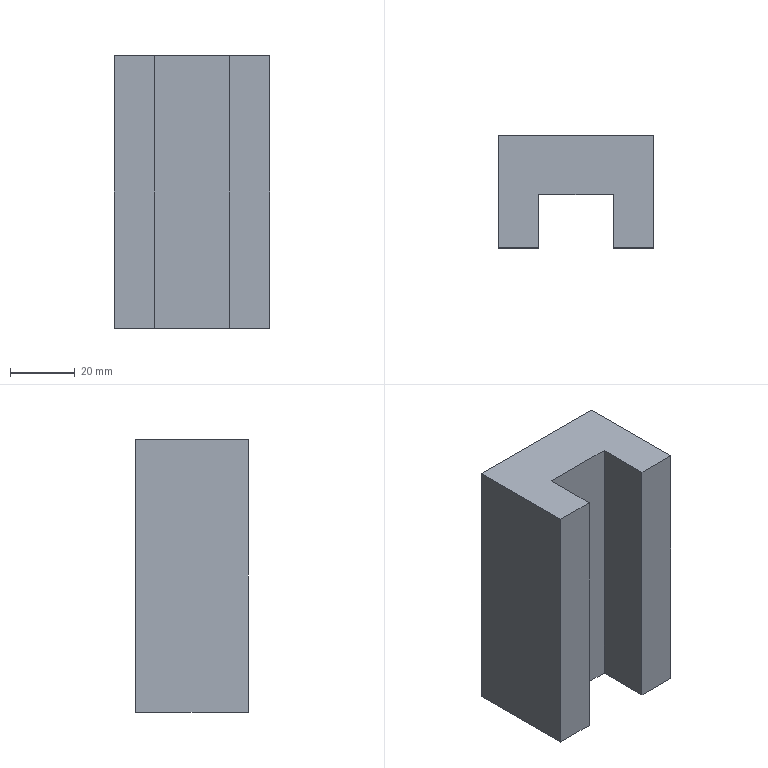Part | SolidWorks | features Extrusion 1, HoleWzd 1 | 1 solid | 26 faces | box 48 x 34.5 x 84 mm | volume 106558 mm3 | plane 10 | cylinder 8 | cone 8 | commonest cylinder face diameters 5 x8
STEP:
#1=CARTESIAN_POINT('',(-17.5,9.25,-20.));
#2=VERTEX_POINT('',#1);
#3=CARTESIAN_POINT('',(-17.5,9.25,-15.));
#4=VERTEX_POINT('',#3);
#5=CARTESIAN_POINT('',(-17.5,9.25,-17.5));
#6=DIRECTION('',(0.,1.,0.));
#7=DIRECTION('',(0.,0.,1.));
#8=AXIS2_PLACEMENT_3D('',#5,#6,#7);
#9=CIRCLE('',#8,2.5);
#10=EDGE_CURVE('',#2,#4,#9,.T.);
#11=ORIENTED_EDGE('',*,*,#10,.F.);
#12=CARTESIAN_POINT('',(-17.5,17.25,-20.));
#13=VERTEX_POINT('',#12);
#14=CARTESIAN_POINT('',(-17.5,17.25,-20.));
#15=DIRECTION('',(0.,1.,0.));
#16=VECTOR('',#15,1000.);
#17=LINE('',#14,#16);
#18=EDGE_CURVE('',#2,#13,#17,.T.);
#19=ORIENTED_EDGE('',*,*,#18,.T.);
#20=CARTESIAN_POINT('',(-17.5,17.25,-15.));
#21=VERTEX_POINT('',#20);
#22=CARTESIAN_POINT('',(-17.5,17.25,-17.5));
#23=DIRECTION('',(0.,1.,0.));
#24=DIRECTION('',(0.,0.,1.));
#25=AXIS2_PLACEMENT_3D('',#22,#23,#24);
#26=CIRCLE('',#25,2.5);
#27=EDGE_CURVE('',#13,#21,#26,.T.);
#28=ORIENTED_EDGE('',*,*,#27,.T.);
#29=CARTESIAN_POINT('',(-17.5,17.25,-15.));
#30=DIRECTION('',(0.,1.,0.));
#31=VECTOR('',#30,1000.);
#32=LINE('',#29,#31);
#33=EDGE_CURVE('',#4,#21,#32,.T.);
#34=ORIENTED_EDGE('',*,*,#33,.F.);
#35=EDGE_LOOP('',(#11,#19,#28,#34));
#36=FACE_OUTER_BOUND('',#35,.T.);
#37=CARTESIAN_POINT('',(-17.5,17.25,-17.5));
#38=DIRECTION('',(0.,1.,0.));
#39=DIRECTION('',(0.,0.,1.));
#40=AXIS2_PLACEMENT_3D('',#37,#38,#39);
#41=CYLINDRICAL_SURFACE('',#40,2.5);
#42=ADVANCED_FACE('',(#36),#41,.F.);
#43=CARTESIAN_POINT('',(-17.5,7.748,-17.5));
#44=VERTEX_POINT('',#43);
#45=CARTESIAN_POINT('',(-17.5,9.25,-15.));
#46=DIRECTION('',(0.,0.515,0.8572));
#47=VECTOR('',#46,1000.);
#48=LINE('',#45,#47);
#49=EDGE_CURVE('',#44,#4,#48,.T.);
#50=ORIENTED_EDGE('',*,*,#49,.F.);
#51=CARTESIAN_POINT('',(-17.5,9.25,-20.));
#52=DIRECTION('',(0.,0.515,-0.8572));
#53=VECTOR('',#52,1000.);
#54=LINE('',#51,#53);
#55=EDGE_CURVE('',#44,#2,#54,.T.);
#56=ORIENTED_EDGE('',*,*,#55,.T.);
#57=ORIENTED_EDGE('',*,*,#10,.T.);
#58=EDGE_LOOP('',(#50,#56,#57));
#59=FACE_OUTER_BOUND('',#58,.T.);
#60=CARTESIAN_POINT('',(-17.5,9.25,-17.5));
#61=DIRECTION('',(0.,1.,0.));
#62=DIRECTION('',(0.,0.,1.));
#63=AXIS2_PLACEMENT_3D('',#60,#61,#62);
#64=CONICAL_SURFACE('',#63,2.5,1.03);
#65=ADVANCED_FACE('',(#59),#64,.F.);
#66=CARTESIAN_POINT('',(17.5,9.25,-20.));
#67=VERTEX_POINT('',#66);
#68=CARTESIAN_POINT('',(17.5,9.25,-15.));
#69=VERTEX_POINT('',#68);
#70=CARTESIAN_POINT('',(17.5,9.25,-17.5));
#71=DIRECTION('',(0.,1.,0.));
#72=DIRECTION('',(0.,0.,1.));
#73=AXIS2_PLACEMENT_3D('',#70,#71,#72);
#74=CIRCLE('',#73,2.5);
#75=EDGE_CURVE('',#67,#69,#74,.T.);
#76=ORIENTED_EDGE('',*,*,#75,.F.);
#77=CARTESIAN_POINT('',(17.5,17.25,-20.));
#78=VERTEX_POINT('',#77);
#79=CARTESIAN_POINT('',(17.5,17.25,-20.));
#80=DIRECTION('',(0.,1.,0.));
#81=VECTOR('',#80,1000.);
#82=LINE('',#79,#81);
#83=EDGE_CURVE('',#67,#78,#82,.T.);
#84=ORIENTED_EDGE('',*,*,#83,.T.);
#85=CARTESIAN_POINT('',(17.5,17.25,-15.));
#86=VERTEX_POINT('',#85);
#87=CARTESIAN_POINT('',(17.5,17.25,-17.5));
#88=DIRECTION('',(0.,1.,0.));
#89=DIRECTION('',(0.,0.,1.));
#90=AXIS2_PLACEMENT_3D('',#87,#88,#89);
#91=CIRCLE('',#90,2.5);
#92=EDGE_CURVE('',#78,#86,#91,.T.);
#93=ORIENTED_EDGE('',*,*,#92,.T.);
#94=CARTESIAN_POINT('',(17.5,17.25,-15.));
#95=DIRECTION('',(0.,1.,0.));
#96=VECTOR('',#95,1000.);
#97=LINE('',#94,#96);
#98=EDGE_CURVE('',#69,#86,#97,.T.);
#99=ORIENTED_EDGE('',*,*,#98,.F.);
#100=EDGE_LOOP('',(#76,#84,#93,#99));
#101=FACE_OUTER_BOUND('',#100,.T.);
#102=CARTESIAN_POINT('',(17.5,17.25,-17.5));
#103=DIRECTION('',(0.,1.,0.));
#104=DIRECTION('',(0.,0.,1.));
#105=AXIS2_PLACEMENT_3D('',#102,#103,#104);
#106=CYLINDRICAL_SURFACE('',#105,2.5);
#107=ADVANCED_FACE('',(#101),#106,.F.);
#108=CARTESIAN_POINT('',(17.5,7.748,-17.5));
#109=VERTEX_POINT('',#108);
#110=CARTESIAN_POINT('',(17.5,9.25,-15.));
#111=DIRECTION('',(0.,0.515,0.8572));
#112=VECTOR('',#111,1000.);
#113=LINE('',#110,#112);
#114=EDGE_CURVE('',#109,#69,#113,.T.);
#115=ORIENTED_EDGE('',*,*,#114,.F.);
#116=CARTESIAN_POINT('',(17.5,9.25,-20.));
#117=DIRECTION('',(0.,0.515,-0.8572));
#118=VECTOR('',#117,1000.);
#119=LINE('',#116,#118);
#120=EDGE_CURVE('',#109,#67,#119,.T.);
#121=ORIENTED_EDGE('',*,*,#120,.T.);
#122=ORIENTED_EDGE('',*,*,#75,.T.);
#123=EDGE_LOOP('',(#115,#121,#122));
#124=FACE_OUTER_BOUND('',#123,.T.);
#125=CARTESIAN_POINT('',(17.5,9.25,-17.5));
#126=DIRECTION('',(0.,1.,0.));
#127=DIRECTION('',(0.,0.,1.));
#128=AXIS2_PLACEMENT_3D('',#125,#126,#127);
#129=CONICAL_SURFACE('',#128,2.5,1.03);
#130=ADVANCED_FACE('',(#124),#129,.F.);
#131=CARTESIAN_POINT('',(17.5,9.25,15.));
#132=VERTEX_POINT('',#131);
#133=CARTESIAN_POINT('',(17.5,9.25,20.));
#134=VERTEX_POINT('',#133);
#135=CARTESIAN_POINT('',(17.5,9.25,17.5));
#136=DIRECTION('',(0.,1.,0.));
#137=DIRECTION('',(0.,0.,1.));
#138=AXIS2_PLACEMENT_3D('',#135,#136,#137);
#139=CIRCLE('',#138,2.5);
#140=EDGE_CURVE('',#132,#134,#139,.T.);
#141=ORIENTED_EDGE('',*,*,#140,.F.);
#142=CARTESIAN_POINT('',(17.5,17.25,15.));
#143=VERTEX_POINT('',#142);
#144=CARTESIAN_POINT('',(17.5,17.25,15.));
#145=DIRECTION('',(0.,1.,0.));
#146=VECTOR('',#145,1000.);
#147=LINE('',#144,#146);
#148=EDGE_CURVE('',#132,#143,#147,.T.);
#149=ORIENTED_EDGE('',*,*,#148,.T.);
#150=CARTESIAN_POINT('',(17.5,17.25,20.));
#151=VERTEX_POINT('',#150);
#152=CARTESIAN_POINT('',(17.5,17.25,17.5));
#153=DIRECTION('',(0.,1.,0.));
#154=DIRECTION('',(0.,0.,1.));
#155=AXIS2_PLACEMENT_3D('',#152,#153,#154);
#156=CIRCLE('',#155,2.5);
#157=EDGE_CURVE('',#143,#151,#156,.T.);
#158=ORIENTED_EDGE('',*,*,#157,.T.);
#159=CARTESIAN_POINT('',(17.5,17.25,20.));
#160=DIRECTION('',(0.,1.,0.));
#161=VECTOR('',#160,1000.);
#162=LINE('',#159,#161);
#163=EDGE_CURVE('',#134,#151,#162,.T.);
#164=ORIENTED_EDGE('',*,*,#163,.F.);
#165=EDGE_LOOP('',(#141,#149,#158,#164));
#166=FACE_OUTER_BOUND('',#165,.T.);
#167=CARTESIAN_POINT('',(17.5,17.25,17.5));
#168=DIRECTION('',(0.,1.,0.));
#169=DIRECTION('',(0.,0.,1.));
#170=AXIS2_PLACEMENT_3D('',#167,#168,#169);
#171=CYLINDRICAL_SURFACE('',#170,2.5);
#172=ADVANCED_FACE('',(#166),#171,.F.);
#173=CARTESIAN_POINT('',(17.5,7.748,17.5));
#174=VERTEX_POINT('',#173);
#175=CARTESIAN_POINT('',(17.5,9.25,20.));
#176=DIRECTION('',(0.,0.515,0.8572));
#177=VECTOR('',#176,1000.);
#178=LINE('',#175,#177);
#179=EDGE_CURVE('',#174,#134,#178,.T.);
#180=ORIENTED_EDGE('',*,*,#179,.F.);
#181=CARTESIAN_POINT('',(17.5,9.25,15.));
#182=DIRECTION('',(0.,0.515,-0.8572));
#183=VECTOR('',#182,1000.);
#184=LINE('',#181,#183);
#185=EDGE_CURVE('',#174,#132,#184,.T.);
#186=ORIENTED_EDGE('',*,*,#185,.T.);
#187=ORIENTED_EDGE('',*,*,#140,.T.);
#188=EDGE_LOOP('',(#180,#186,#187));
#189=FACE_OUTER_BOUND('',#188,.T.);
#190=CARTESIAN_POINT('',(17.5,9.25,17.5));
#191=DIRECTION('',(0.,1.,0.));
#192=DIRECTION('',(0.,0.,1.));
#193=AXIS2_PLACEMENT_3D('',#190,#191,#192);
#194=CONICAL_SURFACE('',#193,2.5,1.03);
#195=ADVANCED_FACE('',(#189),#194,.F.);
#196=CARTESIAN_POINT('',(-17.5,9.25,15.));
#197=VERTEX_POINT('',#196);
#198=CARTESIAN_POINT('',(-17.5,9.25,20.));
#199=VERTEX_POINT('',#198);
#200=CARTESIAN_POINT('',(-17.5,9.25,17.5));
#201=DIRECTION('',(0.,1.,0.));
#202=DIRECTION('',(0.,0.,1.));
#203=AXIS2_PLACEMENT_3D('',#200,#201,#202);
#204=CIRCLE('',#203,2.5);
#205=EDGE_CURVE('',#197,#199,#204,.T.);
#206=ORIENTED_EDGE('',*,*,#205,.F.);
#207=CARTESIAN_POINT('',(-17.5,17.25,15.));
#208=VERTEX_POINT('',#207);
#209=CARTESIAN_POINT('',(-17.5,17.25,15.));
#210=DIRECTION('',(0.,1.,0.));
#211=VECTOR('',#210,1000.);
#212=LINE('',#209,#211);
#213=EDGE_CURVE('',#197,#208,#212,.T.);
#214=ORIENTED_EDGE('',*,*,#213,.T.);
#215=CARTESIAN_POINT('',(-17.5,17.25,20.));
#216=VERTEX_POINT('',#215);
#217=CARTESIAN_POINT('',(-17.5,17.25,17.5));
#218=DIRECTION('',(0.,1.,0.));
#219=DIRECTION('',(0.,0.,1.));
#220=AXIS2_PLACEMENT_3D('',#217,#218,#219);
#221=CIRCLE('',#220,2.5);
#222=EDGE_CURVE('',#208,#216,#221,.T.);
#223=ORIENTED_EDGE('',*,*,#222,.T.);
#224=CARTESIAN_POINT('',(-17.5,17.25,20.));
#225=DIRECTION('',(0.,1.,0.));
#226=VECTOR('',#225,1000.);
#227=LINE('',#224,#226);
#228=EDGE_CURVE('',#199,#216,#227,.T.);
#229=ORIENTED_EDGE('',*,*,#228,.F.);
#230=EDGE_LOOP('',(#206,#214,#223,#229));
#231=FACE_OUTER_BOUND('',#230,.T.);
#232=CARTESIAN_POINT('',(-17.5,17.25,17.5));
#233=DIRECTION('',(0.,1.,0.));
#234=DIRECTION('',(0.,0.,1.));
#235=AXIS2_PLACEMENT_3D('',#232,#233,#234);
#236=CYLINDRICAL_SURFACE('',#235,2.5);
#237=ADVANCED_FACE('',(#231),#236,.F.);
#238=CARTESIAN_POINT('',(-17.5,7.748,17.5));
#239=VERTEX_POINT('',#238);
#240=CARTESIAN_POINT('',(-17.5,9.25,20.));
#241=DIRECTION('',(0.,0.515,0.8572));
#242=VECTOR('',#241,1000.);
#243=LINE('',#240,#242);
#244=EDGE_CURVE('',#239,#199,#243,.T.);
#245=ORIENTED_EDGE('',*,*,#244,.F.);
#246=CARTESIAN_POINT('',(-17.5,9.25,15.));
#247=DIRECTION('',(0.,0.515,-0.8572));
#248=VECTOR('',#247,1000.);
#249=LINE('',#246,#248);
#250=EDGE_CURVE('',#239,#197,#249,.T.);
#251=ORIENTED_EDGE('',*,*,#250,.T.);
#252=ORIENTED_EDGE('',*,*,#205,.T.);
#253=EDGE_LOOP('',(#245,#251,#252));
#254=FACE_OUTER_BOUND('',#253,.T.);
#255=CARTESIAN_POINT('',(-17.5,9.25,17.5));
#256=DIRECTION('',(0.,1.,0.));
#257=DIRECTION('',(0.,0.,1.));
#258=AXIS2_PLACEMENT_3D('',#255,#256,#257);
#259=CONICAL_SURFACE('',#258,2.5,1.03);
#260=ADVANCED_FACE('',(#254),#259,.F.);
#261=CARTESIAN_POINT('',(-24.,17.25,-42.));
#262=VERTEX_POINT('',#261);
#263=CARTESIAN_POINT('',(-24.,-17.25,-42.));
#264=VERTEX_POINT('',#263);
#265=CARTESIAN_POINT('',(-24.,-17.25,-42.));
#266=DIRECTION('',(0.,-1.,0.));
#267=VECTOR('',#266,1000.);
#268=LINE('',#265,#267);
#269=EDGE_CURVE('',#262,#264,#268,.T.);
#270=ORIENTED_EDGE('',*,*,#269,.T.);
#271=CARTESIAN_POINT('',(-24.,-17.25,42.));
#272=VERTEX_POINT('',#271);
#273=CARTESIAN_POINT('',(-24.,-17.25,42.));
#274=DIRECTION('',(0.,0.,-1.));
#275=VECTOR('',#274,1000.);
#276=LINE('',#273,#275);
#277=EDGE_CURVE('',#272,#264,#276,.T.);
#278=ORIENTED_EDGE('',*,*,#277,.F.);
#279=CARTESIAN_POINT('',(-24.,17.25,42.));
#280=VERTEX_POINT('',#279);
#281=CARTESIAN_POINT('',(-24.,-17.25,42.));
#282=DIRECTION('',(0.,-1.,0.));
#283=VECTOR('',#282,1000.);
#284=LINE('',#281,#283);
#285=EDGE_CURVE('',#280,#272,#284,.T.);
#286=ORIENTED_EDGE('',*,*,#285,.F.);
#287=CARTESIAN_POINT('',(-24.,17.25,42.));
#288=DIRECTION('',(0.,0.,-1.));
#289=VECTOR('',#288,1000.);
#290=LINE('',#287,#289);
#291=EDGE_CURVE('',#280,#262,#290,.T.);
#292=ORIENTED_EDGE('',*,*,#291,.T.);
#293=EDGE_LOOP('',(#270,#278,#286,#292));
#294=FACE_OUTER_BOUND('',#293,.T.);
#295=CARTESIAN_POINT('',(-24.,-17.25,42.));
#296=DIRECTION('',(1.,0.,0.));
#297=DIRECTION('',(0.,0.,-1.));
#298=AXIS2_PLACEMENT_3D('',#295,#296,#297);
#299=PLANE('',#298);
#300=ADVANCED_FACE('',(#294),#299,.F.);
#301=CARTESIAN_POINT('',(-11.5,-17.25,-42.));
#302=VERTEX_POINT('',#301);
#303=CARTESIAN_POINT('',(-11.5,-17.25,-42.));
#304=DIRECTION('',(1.,0.,0.));
#305=VECTOR('',#304,1000.);
#306=LINE('',#303,#305);
#307=EDGE_CURVE('',#264,#302,#306,.T.);
#308=ORIENTED_EDGE('',*,*,#307,.T.);
#309=CARTESIAN_POINT('',(-11.5,-17.25,42.));
#310=VERTEX_POINT('',#309);
#311=CARTESIAN_POINT('',(-11.5,-17.25,42.));
#312=DIRECTION('',(0.,0.,-1.));
#313=VECTOR('',#312,1000.);
#314=LINE('',#311,#313);
#315=EDGE_CURVE('',#310,#302,#314,.T.);
#316=ORIENTED_EDGE('',*,*,#315,.F.);
#317=CARTESIAN_POINT('',(-11.5,-17.25,42.));
#318=DIRECTION('',(1.,0.,0.));
#319=VECTOR('',#318,1000.);
#320=LINE('',#317,#319);
#321=EDGE_CURVE('',#272,#310,#320,.T.);
#322=ORIENTED_EDGE('',*,*,#321,.F.);
#323=ORIENTED_EDGE('',*,*,#277,.T.);
#324=EDGE_LOOP('',(#308,#316,#322,#323));
#325=FACE_OUTER_BOUND('',#324,.T.);
#326=CARTESIAN_POINT('',(-11.5,-17.25,42.));
#327=DIRECTION('',(0.,1.,0.));
#328=DIRECTION('',(0.,0.,1.));
#329=AXIS2_PLACEMENT_3D('',#326,#327,#328);
#330=PLANE('',#329);
#331=ADVANCED_FACE('',(#325),#330,.F.);
#332=CARTESIAN_POINT('',(-11.5,-0.75,-42.));
#333=VERTEX_POINT('',#332);
#334=CARTESIAN_POINT('',(-11.5,-0.75,-42.));
#335=DIRECTION('',(0.,1.,0.));
#336=VECTOR('',#335,1000.);
#337=LINE('',#334,#336);
#338=EDGE_CURVE('',#302,#333,#337,.T.);
#339=ORIENTED_EDGE('',*,*,#338,.T.);
#340=CARTESIAN_POINT('',(-11.5,-0.75,42.));
#341=VERTEX_POINT('',#340);
#342=CARTESIAN_POINT('',(-11.5,-0.75,42.));
#343=DIRECTION('',(0.,0.,-1.));
#344=VECTOR('',#343,1000.);
#345=LINE('',#342,#344);
#346=EDGE_CURVE('',#341,#333,#345,.T.);
#347=ORIENTED_EDGE('',*,*,#346,.F.);
#348=CARTESIAN_POINT('',(-11.5,-0.75,42.));
#349=DIRECTION('',(0.,1.,0.));
#350=VECTOR('',#349,1000.);
#351=LINE('',#348,#350);
#352=EDGE_CURVE('',#310,#341,#351,.T.);
#353=ORIENTED_EDGE('',*,*,#352,.F.);
#354=ORIENTED_EDGE('',*,*,#315,.T.);
#355=EDGE_LOOP('',(#339,#347,#353,#354));
#356=FACE_OUTER_BOUND('',#355,.T.);
#357=CARTESIAN_POINT('',(-11.5,-0.75,42.));
#358=DIRECTION('',(-1.,0.,0.));
#359=DIRECTION('',(0.,-1.,0.));
#360=AXIS2_PLACEMENT_3D('',#357,#358,#359);
#361=PLANE('',#360);
#362=ADVANCED_FACE('',(#356),#361,.F.);
#363=CARTESIAN_POINT('',(11.5,-0.75,-42.));
#364=VERTEX_POINT('',#363);
#365=CARTESIAN_POINT('',(-11.5,-0.75,-42.));
#366=DIRECTION('',(1.,0.,0.));
#367=VECTOR('',#366,1000.);
#368=LINE('',#365,#367);
#369=EDGE_CURVE('',#333,#364,#368,.T.);
#370=ORIENTED_EDGE('',*,*,#369,.T.);
#371=CARTESIAN_POINT('',(11.5,-0.75,42.));
#372=VERTEX_POINT('',#371);
#373=CARTESIAN_POINT('',(11.5,-0.75,42.));
#374=DIRECTION('',(0.,0.,-1.));
#375=VECTOR('',#374,1000.);
#376=LINE('',#373,#375);
#377=EDGE_CURVE('',#372,#364,#376,.T.);
#378=ORIENTED_EDGE('',*,*,#377,.F.);
#379=CARTESIAN_POINT('',(-11.5,-0.75,42.));
#380=DIRECTION('',(1.,0.,0.));
#381=VECTOR('',#380,1000.);
#382=LINE('',#379,#381);
#383=EDGE_CURVE('',#341,#372,#382,.T.);
#384=ORIENTED_EDGE('',*,*,#383,.F.);
#385=ORIENTED_EDGE('',*,*,#346,.T.);
#386=EDGE_LOOP('',(#370,#378,#384,#385));
#387=FACE_OUTER_BOUND('',#386,.T.);
#388=CARTESIAN_POINT('',(-11.5,-0.75,42.));
#389=DIRECTION('',(0.,1.,0.));
#390=DIRECTION('',(-1.,0.,0.));
#391=AXIS2_PLACEMENT_3D('',#388,#389,#390);
#392=PLANE('',#391);
#393=ADVANCED_FACE('',(#387),#392,.F.);
#394=CARTESIAN_POINT('',(11.5,-17.25,-42.));
#395=VERTEX_POINT('',#394);
#396=CARTESIAN_POINT('',(11.5,-0.75,-42.));
#397=DIRECTION('',(0.,-1.,0.));
#398=VECTOR('',#397,1000.);
#399=LINE('',#396,#398);
#400=EDGE_CURVE('',#364,#395,#399,.T.);
#401=ORIENTED_EDGE('',*,*,#400,.T.);
#402=CARTESIAN_POINT('',(11.5,-17.25,42.));
#403=VERTEX_POINT('',#402);
#404=CARTESIAN_POINT('',(11.5,-17.25,42.));
#405=DIRECTION('',(0.,0.,-1.));
#406=VECTOR('',#405,1000.);
#407=LINE('',#404,#406);
#408=EDGE_CURVE('',#403,#395,#407,.T.);
#409=ORIENTED_EDGE('',*,*,#408,.F.);
#410=CARTESIAN_POINT('',(11.5,-0.75,42.));
#411=DIRECTION('',(0.,-1.,0.));
#412=VECTOR('',#411,1000.);
#413=LINE('',#410,#412);
#414=EDGE_CURVE('',#372,#403,#413,.T.);
#415=ORIENTED_EDGE('',*,*,#414,.F.);
#416=ORIENTED_EDGE('',*,*,#377,.T.);
#417=EDGE_LOOP('',(#401,#409,#415,#416));
#418=FACE_OUTER_BOUND('',#417,.T.);
#419=CARTESIAN_POINT('',(11.5,-0.75,42.));
#420=DIRECTION('',(1.,0.,0.));
#421=DIRECTION('',(0.,1.,0.));
#422=AXIS2_PLACEMENT_3D('',#419,#420,#421);
#423=PLANE('',#422);
#424=ADVANCED_FACE('',(#418),#423,.F.);
#425=CARTESIAN_POINT('',(24.,-17.25,-42.));
#426=VERTEX_POINT('',#425);
#427=CARTESIAN_POINT('',(24.,-17.25,-42.));
#428=DIRECTION('',(1.,0.,0.));
#429=VECTOR('',#428,1000.);
#430=LINE('',#427,#429);
#431=EDGE_CURVE('',#395,#426,#430,.T.);
#432=ORIENTED_EDGE('',*,*,#431,.T.);
#433=CARTESIAN_POINT('',(24.,-17.25,42.));
#434=VERTEX_POINT('',#433);
#435=CARTESIAN_POINT('',(24.,-17.25,42.));
#436=DIRECTION('',(0.,0.,-1.));
#437=VECTOR('',#436,1000.);
#438=LINE('',#435,#437);
#439=EDGE_CURVE('',#434,#426,#438,.T.);
#440=ORIENTED_EDGE('',*,*,#439,.F.);
#441=CARTESIAN_POINT('',(24.,-17.25,42.));
#442=DIRECTION('',(1.,0.,0.));
#443=VECTOR('',#442,1000.);
#444=LINE('',#441,#443);
#445=EDGE_CURVE('',#403,#434,#444,.T.);
#446=ORIENTED_EDGE('',*,*,#445,.F.);
#447=ORIENTED_EDGE('',*,*,#408,.T.);
#448=EDGE_LOOP('',(#432,#440,#446,#447));
#449=FACE_OUTER_BOUND('',#448,.T.);
#450=CARTESIAN_POINT('',(24.,-17.25,42.));
#451=DIRECTION('',(0.,1.,0.));
#452=DIRECTION('',(-1.,0.,0.));
#453=AXIS2_PLACEMENT_3D('',#450,#451,#452);
#454=PLANE('',#453);
#455=ADVANCED_FACE('',(#449),#454,.F.);
#456=CARTESIAN_POINT('',(24.,17.25,-42.));
#457=VERTEX_POINT('',#456);
#458=CARTESIAN_POINT('',(24.,-17.25,-42.));
#459=DIRECTION('',(0.,1.,0.));
#460=VECTOR('',#459,1000.);
#461=LINE('',#458,#460);
#462=EDGE_CURVE('',#426,#457,#461,.T.);
#463=ORIENTED_EDGE('',*,*,#462,.T.);
#464=CARTESIAN_POINT('',(24.,17.25,42.));
#465=VERTEX_POINT('',#464);
#466=CARTESIAN_POINT('',(24.,17.25,42.));
#467=DIRECTION('',(0.,0.,-1.));
#468=VECTOR('',#467,1000.);
#469=LINE('',#466,#468);
#470=EDGE_CURVE('',#465,#457,#469,.T.);
#471=ORIENTED_EDGE('',*,*,#470,.F.);
#472=CARTESIAN_POINT('',(24.,-17.25,42.));
#473=DIRECTION('',(0.,1.,0.));
#474=VECTOR('',#473,1000.);
#475=LINE('',#472,#474);
#476=EDGE_CURVE('',#434,#465,#475,.T.);
#477=ORIENTED_EDGE('',*,*,#476,.F.);
#478=ORIENTED_EDGE('',*,*,#439,.T.);
#479=EDGE_LOOP('',(#463,#471,#477,#478));
#480=FACE_OUTER_BOUND('',#479,.T.);
#481=CARTESIAN_POINT('',(24.,-17.25,42.));
#482=DIRECTION('',(-1.,0.,0.));
#483=DIRECTION('',(0.,0.,1.));
#484=AXIS2_PLACEMENT_3D('',#481,#482,#483);
#485=PLANE('',#484);
#486=ADVANCED_FACE('',(#480),#485,.F.);
#487=CARTESIAN_POINT('',(-17.5,17.25,-17.5));
#488=DIRECTION('',(0.,1.,0.));
#489=DIRECTION('',(0.,0.,1.));
#490=AXIS2_PLACEMENT_3D('',#487,#488,#489);
#491=CIRCLE('',#490,2.5);
#492=EDGE_CURVE('',#21,#13,#491,.T.);
#493=ORIENTED_EDGE('',*,*,#492,.F.);
#494=ORIENTED_EDGE('',*,*,#27,.F.);
#495=EDGE_LOOP('',(#493,#494));
#496=FACE_BOUND('',#495,.T.);
#497=CARTESIAN_POINT('',(17.5,17.25,-17.5));
#498=DIRECTION('',(0.,1.,0.));
#499=DIRECTION('',(0.,0.,1.));
#500=AXIS2_PLACEMENT_3D('',#497,#498,#499);
#501=CIRCLE('',#500,2.5);
#502=EDGE_CURVE('',#86,#78,#501,.T.);
#503=ORIENTED_EDGE('',*,*,#502,.F.);
#504=ORIENTED_EDGE('',*,*,#92,.F.);
#505=EDGE_LOOP('',(#503,#504));
#506=FACE_BOUND('',#505,.T.);
#507=CARTESIAN_POINT('',(17.5,17.25,17.5));
#508=DIRECTION('',(0.,1.,0.));
#509=DIRECTION('',(0.,0.,1.));
#510=AXIS2_PLACEMENT_3D('',#507,#508,#509);
#511=CIRCLE('',#510,2.5);
#512=EDGE_CURVE('',#151,#143,#511,.T.);
#513=ORIENTED_EDGE('',*,*,#512,.F.);
#514=ORIENTED_EDGE('',*,*,#157,.F.);
#515=EDGE_LOOP('',(#513,#514));
#516=FACE_BOUND('',#515,.T.);
#517=CARTESIAN_POINT('',(-17.5,17.25,17.5));
#518=DIRECTION('',(0.,1.,0.));
#519=DIRECTION('',(0.,0.,1.));
#520=AXIS2_PLACEMENT_3D('',#517,#518,#519);
#521=CIRCLE('',#520,2.5);
#522=EDGE_CURVE('',#216,#208,#521,.T.);
#523=ORIENTED_EDGE('',*,*,#522,.F.);
#524=ORIENTED_EDGE('',*,*,#222,.F.);
#525=EDGE_LOOP('',(#523,#524));
#526=FACE_BOUND('',#525,.T.);
#527=CARTESIAN_POINT('',(24.,17.25,-42.));
#528=DIRECTION('',(-1.,0.,0.));
#529=VECTOR('',#528,1000.);
#530=LINE('',#527,#529);
#531=EDGE_CURVE('',#457,#262,#530,.T.);
#532=ORIENTED_EDGE('',*,*,#531,.T.);
#533=ORIENTED_EDGE('',*,*,#291,.F.);
#534=CARTESIAN_POINT('',(24.,17.25,42.));
#535=DIRECTION('',(-1.,0.,0.));
#536=VECTOR('',#535,1000.);
#537=LINE('',#534,#536);
#538=EDGE_CURVE('',#465,#280,#537,.T.);
#539=ORIENTED_EDGE('',*,*,#538,.F.);
#540=ORIENTED_EDGE('',*,*,#470,.T.);
#541=EDGE_LOOP('',(#532,#533,#539,#540));
#542=FACE_OUTER_BOUND('',#541,.T.);
#543=CARTESIAN_POINT('',(24.,17.25,42.));
#544=DIRECTION('',(0.,-1.,0.));
#545=DIRECTION('',(1.,0.,0.));
#546=AXIS2_PLACEMENT_3D('',#543,#544,#545);
#547=PLANE('',#546);
#548=ADVANCED_FACE('',(#496,#506,#516,#526,#542),#547,.F.);
#549=ORIENTED_EDGE('',*,*,#285,.T.);
#550=ORIENTED_EDGE('',*,*,#321,.T.);
#551=ORIENTED_EDGE('',*,*,#352,.T.);
#552=ORIENTED_EDGE('',*,*,#383,.T.);
#553=ORIENTED_EDGE('',*,*,#414,.T.);
#554=ORIENTED_EDGE('',*,*,#445,.T.);
#555=ORIENTED_EDGE('',*,*,#476,.T.);
#556=ORIENTED_EDGE('',*,*,#538,.T.);
#557=EDGE_LOOP('',(#549,#550,#551,#552,#553,#554,#555,#556));
#558=FACE_OUTER_BOUND('',#557,.T.);
#559=CARTESIAN_POINT('',(0.,0.,42.));
#560=DIRECTION('',(0.,0.,1.));
#561=DIRECTION('',(1.,0.,0.));
#562=AXIS2_PLACEMENT_3D('',#559,#560,#561);
#563=PLANE('',#562);
#564=ADVANCED_FACE('',(#558),#563,.T.);
#565=ORIENTED_EDGE('',*,*,#269,.F.);
#566=ORIENTED_EDGE('',*,*,#531,.F.);
#567=ORIENTED_EDGE('',*,*,#462,.F.);
#568=ORIENTED_EDGE('',*,*,#431,.F.);
#569=ORIENTED_EDGE('',*,*,#400,.F.);
#570=ORIENTED_EDGE('',*,*,#369,.F.);
#571=ORIENTED_EDGE('',*,*,#338,.F.);
#572=ORIENTED_EDGE('',*,*,#307,.F.);
#573=EDGE_LOOP('',(#565,#566,#567,#568,#569,#570,#571,#572));
#574=FACE_OUTER_BOUND('',#573,.T.);
#575=CARTESIAN_POINT('',(0.,0.,-42.));
#576=DIRECTION('',(0.,0.,1.));
#577=DIRECTION('',(1.,0.,0.));
#578=AXIS2_PLACEMENT_3D('',#575,#576,#577);
#579=PLANE('',#578);
#580=ADVANCED_FACE('',(#574),#579,.F.);
#581=ORIENTED_EDGE('',*,*,#250,.F.);
#582=ORIENTED_EDGE('',*,*,#244,.T.);
#583=CARTESIAN_POINT('',(-17.5,9.25,17.5));
#584=DIRECTION('',(0.,1.,0.));
#585=DIRECTION('',(0.,0.,1.));
#586=AXIS2_PLACEMENT_3D('',#583,#584,#585);
#587=CIRCLE('',#586,2.5);
#588=EDGE_CURVE('',#199,#197,#587,.T.);
#589=ORIENTED_EDGE('',*,*,#588,.T.);
#590=EDGE_LOOP('',(#581,#582,#589));
#591=FACE_OUTER_BOUND('',#590,.T.);
#592=CARTESIAN_POINT('',(-17.5,9.25,17.5));
#593=DIRECTION('',(0.,1.,0.));
#594=DIRECTION('',(0.,0.,1.));
#595=AXIS2_PLACEMENT_3D('',#592,#593,#594);
#596=CONICAL_SURFACE('',#595,2.5,1.03);
#597=ADVANCED_FACE('',(#591),#596,.F.);
#598=ORIENTED_EDGE('',*,*,#213,.F.);
#599=ORIENTED_EDGE('',*,*,#588,.F.);
#600=ORIENTED_EDGE('',*,*,#228,.T.);
#601=ORIENTED_EDGE('',*,*,#522,.T.);
#602=EDGE_LOOP('',(#598,#599,#600,#601));
#603=FACE_OUTER_BOUND('',#602,.T.);
#604=CARTESIAN_POINT('',(-17.5,17.25,17.5));
#605=DIRECTION('',(0.,1.,0.));
#606=DIRECTION('',(0.,0.,1.));
#607=AXIS2_PLACEMENT_3D('',#604,#605,#606);
#608=CYLINDRICAL_SURFACE('',#607,2.5);
#609=ADVANCED_FACE('',(#603),#608,.F.);
#610=ORIENTED_EDGE('',*,*,#185,.F.);
#611=ORIENTED_EDGE('',*,*,#179,.T.);
#612=CARTESIAN_POINT('',(17.5,9.25,17.5));
#613=DIRECTION('',(0.,1.,0.));
#614=DIRECTION('',(0.,0.,1.));
#615=AXIS2_PLACEMENT_3D('',#612,#613,#614);
#616=CIRCLE('',#615,2.5);
#617=EDGE_CURVE('',#134,#132,#616,.T.);
#618=ORIENTED_EDGE('',*,*,#617,.T.);
#619=EDGE_LOOP('',(#610,#611,#618));
#620=FACE_OUTER_BOUND('',#619,.T.);
#621=CARTESIAN_POINT('',(17.5,9.25,17.5));
#622=DIRECTION('',(0.,1.,0.));
#623=DIRECTION('',(0.,0.,1.));
#624=AXIS2_PLACEMENT_3D('',#621,#622,#623);
#625=CONICAL_SURFACE('',#624,2.5,1.03);
#626=ADVANCED_FACE('',(#620),#625,.F.);
#627=ORIENTED_EDGE('',*,*,#148,.F.);
#628=ORIENTED_EDGE('',*,*,#617,.F.);
#629=ORIENTED_EDGE('',*,*,#163,.T.);
#630=ORIENTED_EDGE('',*,*,#512,.T.);
#631=EDGE_LOOP('',(#627,#628,#629,#630));
#632=FACE_OUTER_BOUND('',#631,.T.);
#633=CARTESIAN_POINT('',(17.5,17.25,17.5));
#634=DIRECTION('',(0.,1.,0.));
#635=DIRECTION('',(0.,0.,1.));
#636=AXIS2_PLACEMENT_3D('',#633,#634,#635);
#637=CYLINDRICAL_SURFACE('',#636,2.5);
#638=ADVANCED_FACE('',(#632),#637,.F.);
#639=ORIENTED_EDGE('',*,*,#120,.F.);
#640=ORIENTED_EDGE('',*,*,#114,.T.);
#641=CARTESIAN_POINT('',(17.5,9.25,-17.5));
#642=DIRECTION('',(0.,1.,0.));
#643=DIRECTION('',(0.,0.,1.));
#644=AXIS2_PLACEMENT_3D('',#641,#642,#643);
#645=CIRCLE('',#644,2.5);
#646=EDGE_CURVE('',#69,#67,#645,.T.);
#647=ORIENTED_EDGE('',*,*,#646,.T.);
#648=EDGE_LOOP('',(#639,#640,#647));
#649=FACE_OUTER_BOUND('',#648,.T.);
#650=CARTESIAN_POINT('',(17.5,9.25,-17.5));
#651=DIRECTION('',(0.,1.,0.));
#652=DIRECTION('',(0.,0.,1.));
#653=AXIS2_PLACEMENT_3D('',#650,#651,#652);
#654=CONICAL_SURFACE('',#653,2.5,1.03);
#655=ADVANCED_FACE('',(#649),#654,.F.);
#656=ORIENTED_EDGE('',*,*,#83,.F.);
#657=ORIENTED_EDGE('',*,*,#646,.F.);
#658=ORIENTED_EDGE('',*,*,#98,.T.);
#659=ORIENTED_EDGE('',*,*,#502,.T.);
#660=EDGE_LOOP('',(#656,#657,#658,#659));
#661=FACE_OUTER_BOUND('',#660,.T.);
#662=CARTESIAN_POINT('',(17.5,17.25,-17.5));
#663=DIRECTION('',(0.,1.,0.));
#664=DIRECTION('',(0.,0.,1.));
#665=AXIS2_PLACEMENT_3D('',#662,#663,#664);
#666=CYLINDRICAL_SURFACE('',#665,2.5);
#667=ADVANCED_FACE('',(#661),#666,.F.);
#668=ORIENTED_EDGE('',*,*,#55,.F.);
#669=ORIENTED_EDGE('',*,*,#49,.T.);
#670=CARTESIAN_POINT('',(-17.5,9.25,-17.5));
#671=DIRECTION('',(0.,1.,0.));
#672=DIRECTION('',(0.,0.,1.));
#673=AXIS2_PLACEMENT_3D('',#670,#671,#672);
#674=CIRCLE('',#673,2.5);
#675=EDGE_CURVE('',#4,#2,#674,.T.);
#676=ORIENTED_EDGE('',*,*,#675,.T.);
#677=EDGE_LOOP('',(#668,#669,#676));
#678=FACE_OUTER_BOUND('',#677,.T.);
#679=CARTESIAN_POINT('',(-17.5,9.25,-17.5));
#680=DIRECTION('',(0.,1.,0.));
#681=DIRECTION('',(0.,0.,1.));
#682=AXIS2_PLACEMENT_3D('',#679,#680,#681);
#683=CONICAL_SURFACE('',#682,2.5,1.03);
#684=ADVANCED_FACE('',(#678),#683,.F.);
#685=ORIENTED_EDGE('',*,*,#18,.F.);
#686=ORIENTED_EDGE('',*,*,#675,.F.);
#687=ORIENTED_EDGE('',*,*,#33,.T.);
#688=ORIENTED_EDGE('',*,*,#492,.T.);
#689=EDGE_LOOP('',(#685,#686,#687,#688));
#690=FACE_OUTER_BOUND('',#689,.T.);
#691=CARTESIAN_POINT('',(-17.5,17.25,-17.5));
#692=DIRECTION('',(0.,1.,0.));
#693=DIRECTION('',(0.,0.,1.));
#694=AXIS2_PLACEMENT_3D('',#691,#692,#693);
#695=CYLINDRICAL_SURFACE('',#694,2.5);
#696=ADVANCED_FACE('',(#690),#695,.F.);
#697=CLOSED_SHELL('',(#42,#65,#107,#130,#172,#195,#237,#260,#300,#331,#362,#393,#424,#455,#486,#548,#564,#580,#597,#609,#626,#638,#655,#667,#684,#696));
#698=MANIFOLD_SOLID_BREP('',#697);
#699=CARTESIAN_POINT('',(0.,0.,0.));
#700=DIRECTION('',(0.,0.,1.));
#701=DIRECTION('',(1.,0.,0.));
#702=AXIS2_PLACEMENT_3D('',#699,#700,#701);
#703=(LENGTH_UNIT()NAMED_UNIT(*)SI_UNIT(.MILLI.,.METRE.));
#704=UNCERTAINTY_MEASURE_WITH_UNIT(LENGTH_MEASURE(0.00001),#703,'','');
#705=(NAMED_UNIT(*)PLANE_ANGLE_UNIT()SI_UNIT($,.RADIAN.));
#706=(NAMED_UNIT(*)SI_UNIT($,.STERADIAN.)SOLID_ANGLE_UNIT());
#707=(GEOMETRIC_REPRESENTATION_CONTEXT(3)GLOBAL_UNCERTAINTY_ASSIGNED_CONTEXT((#704))GLOBAL_UNIT_ASSIGNED_CONTEXT((#703,#705,#706))REPRESENTATION_CONTEXT('',''));
#708=ADVANCED_BREP_SHAPE_REPRESENTATION('',(#698,#702),#707);